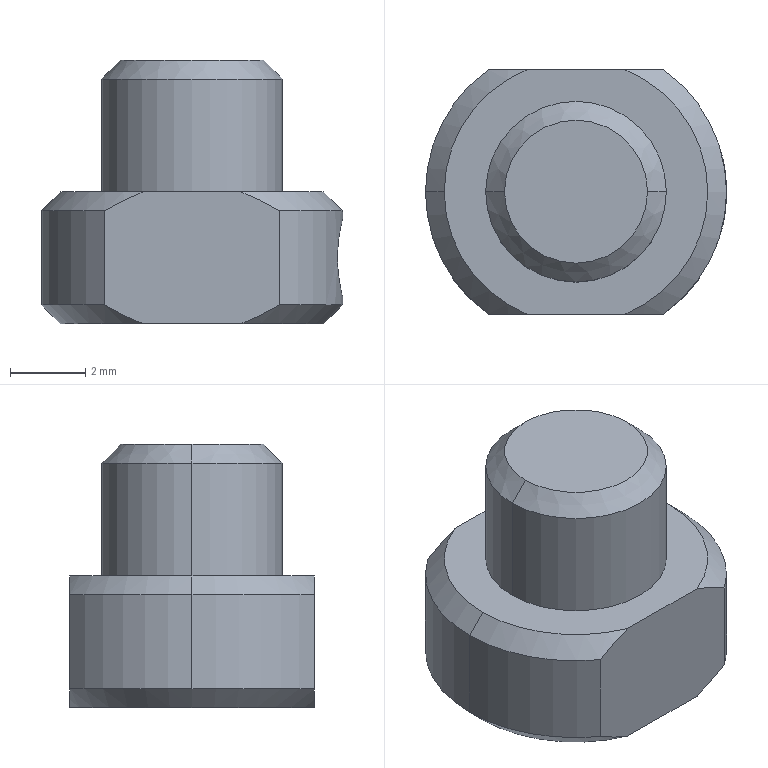Part | SolidWorks | features ICE 3, Chamfer 1, Extrusion 1, HoleWzd 1 | 1 solid | 23 faces | box 8 x 6.5 x 7 mm | volume 166.104 mm3 | cylinder 9 | cone 8 | plane 6 | commonest cylinder face diameters 8 x3 2.05 x2 3 x2 4.8 x2
STEP:
#1=CARTESIAN_POINT('',(1.9,0.,7.));
#2=VERTEX_POINT('',#1);
#3=CARTESIAN_POINT('',(-1.9,0.,7.));
#4=VERTEX_POINT('',#3);
#5=CARTESIAN_POINT('',(0.,0.,7.));
#6=DIRECTION('',(0.,0.,1.));
#7=DIRECTION('',(1.,0.,0.));
#8=AXIS2_PLACEMENT_3D('',#5,#6,#7);
#9=CIRCLE('',#8,1.9);
#10=EDGE_CURVE('',#2,#4,#9,.T.);
#11=ORIENTED_EDGE('',*,*,#10,.F.);
#12=CARTESIAN_POINT('',(2.4,0.,6.5));
#13=VERTEX_POINT('',#12);
#14=CARTESIAN_POINT('',(1.9,0.,7.));
#15=DIRECTION('',(0.7071,0.,-0.7071));
#16=VECTOR('',#15,1000.);
#17=LINE('',#14,#16);
#18=EDGE_CURVE('',#2,#13,#17,.T.);
#19=ORIENTED_EDGE('',*,*,#18,.T.);
#20=CARTESIAN_POINT('',(-2.4,0.,6.5));
#21=VERTEX_POINT('',#20);
#22=CARTESIAN_POINT('',(0.,0.,6.5));
#23=DIRECTION('',(0.,0.,-1.));
#24=DIRECTION('',(1.,0.,0.));
#25=AXIS2_PLACEMENT_3D('',#22,#23,#24);
#26=CIRCLE('',#25,2.4);
#27=EDGE_CURVE('',#21,#13,#26,.T.);
#28=ORIENTED_EDGE('',*,*,#27,.F.);
#29=CARTESIAN_POINT('',(-1.9,0.,7.));
#30=DIRECTION('',(-0.7071,0.,-0.7071));
#31=VECTOR('',#30,1000.);
#32=LINE('',#29,#31);
#33=EDGE_CURVE('',#4,#21,#32,.T.);
#34=ORIENTED_EDGE('',*,*,#33,.F.);
#35=EDGE_LOOP('',(#11,#19,#28,#34));
#36=FACE_OUTER_BOUND('',#35,.T.);
#37=CARTESIAN_POINT('',(0.,0.,7.));
#38=DIRECTION('',(0.,0.,-1.));
#39=DIRECTION('',(-1.,0.,0.));
#40=AXIS2_PLACEMENT_3D('',#37,#38,#39);
#41=CONICAL_SURFACE('',#40,1.9,0.7854);
#42=ADVANCED_FACE('',(#36),#41,.T.);
#43=CARTESIAN_POINT('',(1.5,0.,2.775));
#44=VERTEX_POINT('',#43);
#45=CARTESIAN_POINT('',(1.5,0.,0.725));
#46=VERTEX_POINT('',#45);
#47=CARTESIAN_POINT('',(1.5,0.,2.775));
#48=CARTESIAN_POINT('',(1.5,-0.1385,2.775));
#49=CARTESIAN_POINT('',(1.48,-0.2773,2.746));
#50=CARTESIAN_POINT('',(1.411,-0.5262,2.64));
#51=CARTESIAN_POINT('',(1.362,-0.6364,2.564));
#52=CARTESIAN_POINT('',(1.261,-0.8192,2.38));
#53=CARTESIAN_POINT('',(1.207,-0.8927,2.271));
#54=CARTESIAN_POINT('',(1.124,-0.9957,2.027));
#55=CARTESIAN_POINT('',(1.095,-1.025,1.889));
#56=CARTESIAN_POINT('',(1.095,-1.025,1.61));
#57=CARTESIAN_POINT('',(1.124,-0.9952,1.471));
#58=CARTESIAN_POINT('',(1.208,-0.8919,1.228));
#59=CARTESIAN_POINT('',(1.262,-0.8179,1.119));
#60=CARTESIAN_POINT('',(1.363,-0.6356,0.9355));
#61=CARTESIAN_POINT('',(1.411,-0.5254,0.8598));
#62=CARTESIAN_POINT('',(1.479,-0.2793,0.7548));
#63=CARTESIAN_POINT('',(1.5,-0.1404,0.725));
#64=CARTESIAN_POINT('',(1.5,0.,0.725));
#65=B_SPLINE_CURVE_WITH_KNOTS('',3,(#47,#48,#49,#50,#51,#52,#53,#54,#55,#56,#57,#58,#59,#60,#61,#62,#63,#64),.UNSPECIFIED.,.F.,.F.,(4,2,2,2,2,2,2,2,4),(0.003321,0.003736,0.00415,0.004565,0.004979,0.005394,0.005808,0.006223,0.006638),.UNSPECIFIED.);
#66=EDGE_CURVE('',#44,#46,#65,.T.);
#67=ORIENTED_EDGE('',*,*,#66,.F.);
#68=CARTESIAN_POINT('',(4.,0.,2.775));
#69=VERTEX_POINT('',#68);
#70=CARTESIAN_POINT('',(4.,0.,2.775));
#71=DIRECTION('',(1.,0.,0.));
#72=VECTOR('',#71,1000.);
#73=LINE('',#70,#72);
#74=EDGE_CURVE('',#44,#69,#73,.T.);
#75=ORIENTED_EDGE('',*,*,#74,.T.);
#76=CARTESIAN_POINT('',(4.,0.,0.725));
#77=VERTEX_POINT('',#76);
#78=CARTESIAN_POINT('',(4.,0.,0.725));
#79=CARTESIAN_POINT('',(4.,-0.1361,0.725));
#80=CARTESIAN_POINT('',(3.993,-0.2695,0.752));
#81=CARTESIAN_POINT('',(3.968,-0.5176,0.8551));
#82=CARTESIAN_POINT('',(3.951,-0.6309,0.9313));
#83=CARTESIAN_POINT('',(3.916,-0.8191,1.12));
#84=CARTESIAN_POINT('',(3.899,-0.8954,1.233));
#85=CARTESIAN_POINT('',(3.874,-0.9977,1.48));
#86=CARTESIAN_POINT('',(3.866,-1.025,1.615));
#87=CARTESIAN_POINT('',(3.866,-1.025,1.884));
#88=CARTESIAN_POINT('',(3.874,-0.9983,2.018));
#89=CARTESIAN_POINT('',(3.899,-0.895,2.267));
#90=CARTESIAN_POINT('',(3.916,-0.8196,2.38));
#91=CARTESIAN_POINT('',(3.951,-0.6297,2.57));
#92=CARTESIAN_POINT('',(3.968,-0.5167,2.645));
#93=CARTESIAN_POINT('',(3.993,-0.2692,2.748));
#94=CARTESIAN_POINT('',(4.,-0.1341,2.775));
#95=CARTESIAN_POINT('',(4.,0.,2.775));
#96=B_SPLINE_CURVE_WITH_KNOTS('',3,(#78,#79,#80,#81,#82,#83,#84,#85,#86,#87,#88,#89,#90,#91,#92,#93,#94,#95),.UNSPECIFIED.,.F.,.F.,(4,2,2,2,2,2,2,2,4),(0.,0.0004023,0.0008045,0.001207,0.001609,0.002011,0.002414,0.002816,0.003218),.UNSPECIFIED.);
#97=EDGE_CURVE('',#77,#69,#96,.T.);
#98=ORIENTED_EDGE('',*,*,#97,.F.);
#99=CARTESIAN_POINT('',(4.,0.,0.725));
#100=DIRECTION('',(1.,0.,0.));
#101=VECTOR('',#100,1000.);
#102=LINE('',#99,#101);
#103=EDGE_CURVE('',#46,#77,#102,.T.);
#104=ORIENTED_EDGE('',*,*,#103,.F.);
#105=EDGE_LOOP('',(#67,#75,#98,#104));
#106=FACE_OUTER_BOUND('',#105,.T.);
#107=CARTESIAN_POINT('',(4.,0.,1.75));
#108=DIRECTION('',(1.,0.,0.));
#109=DIRECTION('',(0.,0.,-1.));
#110=AXIS2_PLACEMENT_3D('',#107,#108,#109);
#111=CYLINDRICAL_SURFACE('',#110,1.025);
#112=ADVANCED_FACE('',(#106),#111,.F.);
#113=CARTESIAN_POINT('',(1.5,0.,6.));
#114=VERTEX_POINT('',#113);
#115=CARTESIAN_POINT('',(-1.5,0.,6.));
#116=VERTEX_POINT('',#115);
#117=CARTESIAN_POINT('',(0.,0.,6.));
#118=DIRECTION('',(0.,0.,-1.));
#119=DIRECTION('',(-1.,0.,0.));
#120=AXIS2_PLACEMENT_3D('',#117,#118,#119);
#121=CIRCLE('',#120,1.5);
#122=EDGE_CURVE('',#114,#116,#121,.T.);
#123=ORIENTED_EDGE('',*,*,#122,.F.);
#124=CARTESIAN_POINT('',(1.5,0.,6.));
#125=DIRECTION('',(0.,0.,-1.));
#126=VECTOR('',#125,1000.);
#127=LINE('',#124,#126);
#128=EDGE_CURVE('',#114,#44,#127,.T.);
#129=ORIENTED_EDGE('',*,*,#128,.T.);
#130=ORIENTED_EDGE('',*,*,#66,.T.);
#131=CARTESIAN_POINT('',(1.5,0.,0.));
#132=VERTEX_POINT('',#131);
#133=CARTESIAN_POINT('',(1.5,0.,6.));
#134=DIRECTION('',(0.,0.,-1.));
#135=VECTOR('',#134,1000.);
#136=LINE('',#133,#135);
#137=EDGE_CURVE('',#46,#132,#136,.T.);
#138=ORIENTED_EDGE('',*,*,#137,.T.);
#139=CARTESIAN_POINT('',(-1.5,0.,0.));
#140=VERTEX_POINT('',#139);
#141=CARTESIAN_POINT('',(0.,0.,0.));
#142=DIRECTION('',(0.,0.,-1.));
#143=DIRECTION('',(-1.,0.,0.));
#144=AXIS2_PLACEMENT_3D('',#141,#142,#143);
#145=CIRCLE('',#144,1.5);
#146=EDGE_CURVE('',#132,#140,#145,.T.);
#147=ORIENTED_EDGE('',*,*,#146,.T.);
#148=CARTESIAN_POINT('',(-1.5,0.,6.));
#149=DIRECTION('',(0.,0.,-1.));
#150=VECTOR('',#149,1000.);
#151=LINE('',#148,#150);
#152=EDGE_CURVE('',#116,#140,#151,.T.);
#153=ORIENTED_EDGE('',*,*,#152,.F.);
#154=EDGE_LOOP('',(#123,#129,#130,#138,#147,#153));
#155=FACE_OUTER_BOUND('',#154,.T.);
#156=CARTESIAN_POINT('',(0.,0.,6.));
#157=DIRECTION('',(0.,0.,-1.));
#158=DIRECTION('',(-1.,0.,0.));
#159=AXIS2_PLACEMENT_3D('',#156,#157,#158);
#160=CYLINDRICAL_SURFACE('',#159,1.5);
#161=ADVANCED_FACE('',(#155),#160,.F.);
#162=ORIENTED_EDGE('',*,*,#27,.T.);
#163=CARTESIAN_POINT('',(2.4,0.,3.5));
#164=VERTEX_POINT('',#163);
#165=CARTESIAN_POINT('',(2.4,0.,7.));
#166=DIRECTION('',(0.,0.,-1.));
#167=VECTOR('',#166,1000.);
#168=LINE('',#165,#167);
#169=EDGE_CURVE('',#13,#164,#168,.T.);
#170=ORIENTED_EDGE('',*,*,#169,.T.);
#171=CARTESIAN_POINT('',(-2.4,0.,3.5));
#172=VERTEX_POINT('',#171);
#173=CARTESIAN_POINT('',(0.,0.,3.5));
#174=DIRECTION('',(0.,0.,1.));
#175=DIRECTION('',(1.,0.,0.));
#176=AXIS2_PLACEMENT_3D('',#173,#174,#175);
#177=CIRCLE('',#176,2.4);
#178=EDGE_CURVE('',#164,#172,#177,.T.);
#179=ORIENTED_EDGE('',*,*,#178,.T.);
#180=CARTESIAN_POINT('',(-2.4,0.,7.));
#181=DIRECTION('',(0.,0.,-1.));
#182=VECTOR('',#181,1000.);
#183=LINE('',#180,#182);
#184=EDGE_CURVE('',#21,#172,#183,.T.);
#185=ORIENTED_EDGE('',*,*,#184,.F.);
#186=EDGE_LOOP('',(#162,#170,#179,#185));
#187=FACE_OUTER_BOUND('',#186,.T.);
#188=CARTESIAN_POINT('',(0.,0.,7.));
#189=DIRECTION('',(0.,0.,-1.));
#190=DIRECTION('',(-1.,0.,0.));
#191=AXIS2_PLACEMENT_3D('',#188,#189,#190);
#192=CYLINDRICAL_SURFACE('',#191,2.4);
#193=ADVANCED_FACE('',(#187),#192,.T.);
#194=CARTESIAN_POINT('',(3.5,0.,0.));
#195=VERTEX_POINT('',#194);
#196=CARTESIAN_POINT('',(1.299,-3.25,0.));
#197=VERTEX_POINT('',#196);
#198=CARTESIAN_POINT('',(0.,0.,0.));
#199=DIRECTION('',(0.,0.,-1.));
#200=DIRECTION('',(1.,0.,0.));
#201=AXIS2_PLACEMENT_3D('',#198,#199,#200);
#202=CIRCLE('',#201,3.5);
#203=EDGE_CURVE('',#195,#197,#202,.T.);
#204=ORIENTED_EDGE('',*,*,#203,.F.);
#205=CARTESIAN_POINT('',(4.,0.,0.5));
#206=VERTEX_POINT('',#205);
#207=CARTESIAN_POINT('',(4.,0.,0.5));
#208=DIRECTION('',(0.7071,0.,0.7071));
#209=VECTOR('',#208,1000.);
#210=LINE('',#207,#209);
#211=EDGE_CURVE('',#195,#206,#210,.T.);
#212=ORIENTED_EDGE('',*,*,#211,.T.);
#213=CARTESIAN_POINT('',(2.332,-3.25,0.5));
#214=VERTEX_POINT('',#213);
#215=CARTESIAN_POINT('',(0.,0.,0.5));
#216=DIRECTION('',(0.,0.,1.));
#217=DIRECTION('',(1.,0.,0.));
#218=AXIS2_PLACEMENT_3D('',#215,#216,#217);
#219=CIRCLE('',#218,4.);
#220=EDGE_CURVE('',#214,#206,#219,.T.);
#221=ORIENTED_EDGE('',*,*,#220,.F.);
#222=CARTESIAN_POINT('',(2.332,-3.25,0.5));
#223=CARTESIAN_POINT('',(2.001,-3.25,0.3069));
#224=CARTESIAN_POINT('',(1.659,-3.25,0.1338));
#225=CARTESIAN_POINT('',(1.299,-3.25,0.));
#226=B_SPLINE_CURVE_WITH_KNOTS('',3,(#222,#223,#224,#225),.UNSPECIFIED.,.F.,.F.,(4,4),(0.007591,0.00874),.UNSPECIFIED.);
#227=EDGE_CURVE('',#214,#197,#226,.T.);
#228=ORIENTED_EDGE('',*,*,#227,.T.);
#229=EDGE_LOOP('',(#204,#212,#221,#228));
#230=FACE_OUTER_BOUND('',#229,.T.);
#231=CARTESIAN_POINT('',(0.,0.,0.5));
#232=DIRECTION('',(0.,0.,1.));
#233=DIRECTION('',(1.,0.,0.));
#234=AXIS2_PLACEMENT_3D('',#231,#232,#233);
#235=CONICAL_SURFACE('',#234,4.,0.7854);
#236=ADVANCED_FACE('',(#230),#235,.T.);
#237=CARTESIAN_POINT('',(-3.5,0.,3.5));
#238=VERTEX_POINT('',#237);
#239=CARTESIAN_POINT('',(-1.299,-3.25,3.5));
#240=VERTEX_POINT('',#239);
#241=CARTESIAN_POINT('',(0.,0.,3.5));
#242=DIRECTION('',(0.,0.,1.));
#243=DIRECTION('',(1.,0.,0.));
#244=AXIS2_PLACEMENT_3D('',#241,#242,#243);
#245=CIRCLE('',#244,3.5);
#246=EDGE_CURVE('',#238,#240,#245,.T.);
#247=ORIENTED_EDGE('',*,*,#246,.F.);
#248=CARTESIAN_POINT('',(-4.,0.,3.));
#249=VERTEX_POINT('',#248);
#250=CARTESIAN_POINT('',(-3.5,0.,3.5));
#251=DIRECTION('',(-0.7071,0.,-0.7071));
#252=VECTOR('',#251,1000.);
#253=LINE('',#250,#252);
#254=EDGE_CURVE('',#238,#249,#253,.T.);
#255=ORIENTED_EDGE('',*,*,#254,.T.);
#256=CARTESIAN_POINT('',(-2.332,-3.25,3.));
#257=VERTEX_POINT('',#256);
#258=CARTESIAN_POINT('',(0.,0.,3.));
#259=DIRECTION('',(0.,0.,-1.));
#260=DIRECTION('',(1.,0.,0.));
#261=AXIS2_PLACEMENT_3D('',#258,#259,#260);
#262=CIRCLE('',#261,4.);
#263=EDGE_CURVE('',#257,#249,#262,.T.);
#264=ORIENTED_EDGE('',*,*,#263,.F.);
#265=CARTESIAN_POINT('',(-2.332,-3.25,3.));
#266=CARTESIAN_POINT('',(-2.001,-3.25,3.193));
#267=CARTESIAN_POINT('',(-1.659,-3.25,3.366));
#268=CARTESIAN_POINT('',(-1.299,-3.25,3.5));
#269=B_SPLINE_CURVE_WITH_KNOTS('',3,(#265,#266,#267,#268),.UNSPECIFIED.,.F.,.F.,(4,4),(0.007591,0.00874),.UNSPECIFIED.);
#270=EDGE_CURVE('',#257,#240,#269,.T.);
#271=ORIENTED_EDGE('',*,*,#270,.T.);
#272=EDGE_LOOP('',(#247,#255,#264,#271));
#273=FACE_OUTER_BOUND('',#272,.T.);
#274=CARTESIAN_POINT('',(0.,0.,3.5));
#275=DIRECTION('',(0.,0.,-1.));
#276=DIRECTION('',(-1.,0.,0.));
#277=AXIS2_PLACEMENT_3D('',#274,#275,#276);
#278=CONICAL_SURFACE('',#277,3.5,0.7854);
#279=ADVANCED_FACE('',(#273),#278,.T.);
#280=ORIENTED_EDGE('',*,*,#263,.T.);
#281=CARTESIAN_POINT('',(-4.,0.,0.5));
#282=VERTEX_POINT('',#281);
#283=CARTESIAN_POINT('',(-4.,0.,3.5));
#284=DIRECTION('',(0.,0.,-1.));
#285=VECTOR('',#284,1000.);
#286=LINE('',#283,#285);
#287=EDGE_CURVE('',#249,#282,#286,.T.);
#288=ORIENTED_EDGE('',*,*,#287,.T.);
#289=CARTESIAN_POINT('',(-2.332,-3.25,0.5));
#290=VERTEX_POINT('',#289);
#291=CARTESIAN_POINT('',(0.,0.,0.5));
#292=DIRECTION('',(0.,0.,1.));
#293=DIRECTION('',(1.,0.,0.));
#294=AXIS2_PLACEMENT_3D('',#291,#292,#293);
#295=CIRCLE('',#294,4.);
#296=EDGE_CURVE('',#282,#290,#295,.T.);
#297=ORIENTED_EDGE('',*,*,#296,.T.);
#298=CARTESIAN_POINT('',(-2.332,-3.25,3.5));
#299=DIRECTION('',(0.,0.,-1.));
#300=VECTOR('',#299,1000.);
#301=LINE('',#298,#300);
#302=EDGE_CURVE('',#257,#290,#301,.T.);
#303=ORIENTED_EDGE('',*,*,#302,.F.);
#304=EDGE_LOOP('',(#280,#288,#297,#303));
#305=FACE_OUTER_BOUND('',#304,.T.);
#306=CARTESIAN_POINT('',(0.,0.,3.5));
#307=DIRECTION('',(0.,0.,-1.));
#308=DIRECTION('',(-1.,0.,0.));
#309=AXIS2_PLACEMENT_3D('',#306,#307,#308);
#310=CYLINDRICAL_SURFACE('',#309,4.);
#311=ADVANCED_FACE('',(#305),#310,.T.);
#312=CARTESIAN_POINT('',(0.,0.,3.5));
#313=DIRECTION('',(0.,0.,1.));
#314=DIRECTION('',(1.,0.,0.));
#315=AXIS2_PLACEMENT_3D('',#312,#313,#314);
#316=CIRCLE('',#315,2.4);
#317=EDGE_CURVE('',#172,#164,#316,.T.);
#318=ORIENTED_EDGE('',*,*,#317,.F.);
#319=ORIENTED_EDGE('',*,*,#178,.F.);
#320=EDGE_LOOP('',(#318,#319));
#321=FACE_BOUND('',#320,.T.);
#322=CARTESIAN_POINT('',(-1.299,3.25,3.5));
#323=VERTEX_POINT('',#322);
#324=CARTESIAN_POINT('',(0.,0.,3.5));
#325=DIRECTION('',(0.,0.,1.));
#326=DIRECTION('',(1.,0.,0.));
#327=AXIS2_PLACEMENT_3D('',#324,#325,#326);
#328=CIRCLE('',#327,3.5);
#329=EDGE_CURVE('',#323,#238,#328,.T.);
#330=ORIENTED_EDGE('',*,*,#329,.T.);
#331=ORIENTED_EDGE('',*,*,#246,.T.);
#332=CARTESIAN_POINT('',(1.299,-3.25,3.5));
#333=VERTEX_POINT('',#332);
#334=CARTESIAN_POINT('',(-5.597,-3.25,3.5));
#335=DIRECTION('',(1.,0.,0.));
#336=VECTOR('',#335,1000.);
#337=LINE('',#334,#336);
#338=EDGE_CURVE('',#240,#333,#337,.T.);
#339=ORIENTED_EDGE('',*,*,#338,.T.);
#340=CARTESIAN_POINT('',(1.299,3.25,3.5));
#341=VERTEX_POINT('',#340);
#342=CARTESIAN_POINT('',(0.,0.,3.5));
#343=DIRECTION('',(0.,0.,1.));
#344=DIRECTION('',(1.,0.,0.));
#345=AXIS2_PLACEMENT_3D('',#342,#343,#344);
#346=CIRCLE('',#345,3.5);
#347=EDGE_CURVE('',#333,#341,#346,.T.);
#348=ORIENTED_EDGE('',*,*,#347,.T.);
#349=CARTESIAN_POINT('',(-5.597,3.25,3.5));
#350=DIRECTION('',(-1.,0.,0.));
#351=VECTOR('',#350,1000.);
#352=LINE('',#349,#351);
#353=EDGE_CURVE('',#341,#323,#352,.T.);
#354=ORIENTED_EDGE('',*,*,#353,.T.);
#355=EDGE_LOOP('',(#330,#331,#339,#348,#354));
#356=FACE_OUTER_BOUND('',#355,.T.);
#357=CARTESIAN_POINT('',(0.,0.,3.5));
#358=DIRECTION('',(0.,0.,1.));
#359=DIRECTION('',(1.,0.,0.));
#360=AXIS2_PLACEMENT_3D('',#357,#358,#359);
#361=PLANE('',#360);
#362=ADVANCED_FACE('',(#321,#356),#361,.T.);
#363=ORIENTED_EDGE('',*,*,#287,.F.);
#364=CARTESIAN_POINT('',(-2.332,3.25,3.));
#365=VERTEX_POINT('',#364);
#366=CARTESIAN_POINT('',(0.,0.,3.));
#367=DIRECTION('',(0.,0.,-1.));
#368=DIRECTION('',(1.,0.,0.));
#369=AXIS2_PLACEMENT_3D('',#366,#367,#368);
#370=CIRCLE('',#369,4.);
#371=EDGE_CURVE('',#249,#365,#370,.T.);
#372=ORIENTED_EDGE('',*,*,#371,.T.);
#373=CARTESIAN_POINT('',(-2.332,3.25,0.5));
#374=VERTEX_POINT('',#373);
#375=CARTESIAN_POINT('',(-2.332,3.25,3.5));
#376=DIRECTION('',(0.,0.,1.));
#377=VECTOR('',#376,1000.);
#378=LINE('',#375,#377);
#379=EDGE_CURVE('',#374,#365,#378,.T.);
#380=ORIENTED_EDGE('',*,*,#379,.F.);
#381=CARTESIAN_POINT('',(0.,0.,0.5));
#382=DIRECTION('',(0.,0.,1.));
#383=DIRECTION('',(1.,0.,0.));
#384=AXIS2_PLACEMENT_3D('',#381,#382,#383);
#385=CIRCLE('',#384,4.);
#386=EDGE_CURVE('',#374,#282,#385,.T.);
#387=ORIENTED_EDGE('',*,*,#386,.T.);
#388=EDGE_LOOP('',(#363,#372,#380,#387));
#389=FACE_OUTER_BOUND('',#388,.T.);
#390=CARTESIAN_POINT('',(0.,0.,3.5));
#391=DIRECTION('',(0.,0.,-1.));
#392=DIRECTION('',(-1.,0.,0.));
#393=AXIS2_PLACEMENT_3D('',#390,#391,#392);
#394=CYLINDRICAL_SURFACE('',#393,4.);
#395=ADVANCED_FACE('',(#389),#394,.T.);
#396=ORIENTED_EDGE('',*,*,#97,.T.);
#397=CARTESIAN_POINT('',(4.,0.,2.775));
#398=CARTESIAN_POINT('',(4.,0.1341,2.775));
#399=CARTESIAN_POINT('',(3.993,0.2695,2.748));
#400=CARTESIAN_POINT('',(3.968,0.5164,2.645));
#401=CARTESIAN_POINT('',(3.951,0.63,2.57));
#402=CARTESIAN_POINT('',(3.916,0.8191,2.381));
#403=CARTESIAN_POINT('',(3.899,0.8945,2.268));
#404=CARTESIAN_POINT('',(3.874,0.9983,2.019));
#405=CARTESIAN_POINT('',(3.866,1.025,1.885));
#406=CARTESIAN_POINT('',(3.866,1.025,1.615));
#407=CARTESIAN_POINT('',(3.874,0.998,1.481));
#408=CARTESIAN_POINT('',(3.899,0.8954,1.233));
#409=CARTESIAN_POINT('',(3.916,0.8192,1.12));
#410=CARTESIAN_POINT('',(3.951,0.6312,0.9315));
#411=CARTESIAN_POINT('',(3.968,0.5175,0.8552));
#412=CARTESIAN_POINT('',(3.993,0.2707,0.7524));
#413=CARTESIAN_POINT('',(4.,0.136,0.725));
#414=CARTESIAN_POINT('',(4.,0.,0.725));
#415=B_SPLINE_CURVE_WITH_KNOTS('',3,(#397,#398,#399,#400,#401,#402,#403,#404,#405,#406,#407,#408,#409,#410,#411,#412,#413,#414),.UNSPECIFIED.,.F.,.F.,(4,2,2,2,2,2,2,2,4),(0.003218,0.00362,0.004022,0.004425,0.004827,0.005229,0.005631,0.006033,0.006435),.UNSPECIFIED.);
#416=EDGE_CURVE('',#69,#77,#415,.T.);
#417=ORIENTED_EDGE('',*,*,#416,.T.);
#418=EDGE_LOOP('',(#396,#417));
#419=FACE_BOUND('',#418,.T.);
#420=CARTESIAN_POINT('',(2.332,-3.25,3.));
#421=VERTEX_POINT('',#420);
#422=CARTESIAN_POINT('',(2.332,-3.25,3.5));
#423=DIRECTION('',(0.,0.,1.));
#424=VECTOR('',#423,1000.);
#425=LINE('',#422,#424);
#426=EDGE_CURVE('',#214,#421,#425,.T.);
#427=ORIENTED_EDGE('',*,*,#426,.F.);
#428=ORIENTED_EDGE('',*,*,#220,.T.);
#429=CARTESIAN_POINT('',(2.332,3.25,0.5));
#430=VERTEX_POINT('',#429);
#431=CARTESIAN_POINT('',(0.,0.,0.5));
#432=DIRECTION('',(0.,0.,1.));
#433=DIRECTION('',(1.,0.,0.));
#434=AXIS2_PLACEMENT_3D('',#431,#432,#433);
#435=CIRCLE('',#434,4.);
#436=EDGE_CURVE('',#206,#430,#435,.T.);
#437=ORIENTED_EDGE('',*,*,#436,.T.);
#438=CARTESIAN_POINT('',(2.332,3.25,3.));
#439=VERTEX_POINT('',#438);
#440=CARTESIAN_POINT('',(2.332,3.25,3.5));
#441=DIRECTION('',(0.,0.,-1.));
#442=VECTOR('',#441,1000.);
#443=LINE('',#440,#442);
#444=EDGE_CURVE('',#439,#430,#443,.T.);
#445=ORIENTED_EDGE('',*,*,#444,.F.);
#446=CARTESIAN_POINT('',(0.,0.,3.));
#447=DIRECTION('',(0.,0.,-1.));
#448=DIRECTION('',(1.,0.,0.));
#449=AXIS2_PLACEMENT_3D('',#446,#447,#448);
#450=CIRCLE('',#449,4.);
#451=EDGE_CURVE('',#439,#421,#450,.T.);
#452=ORIENTED_EDGE('',*,*,#451,.T.);
#453=EDGE_LOOP('',(#427,#428,#437,#445,#452));
#454=FACE_OUTER_BOUND('',#453,.T.);
#455=CARTESIAN_POINT('',(0.,0.,3.5));
#456=DIRECTION('',(0.,0.,-1.));
#457=DIRECTION('',(-1.,0.,0.));
#458=AXIS2_PLACEMENT_3D('',#455,#456,#457);
#459=CYLINDRICAL_SURFACE('',#458,4.);
#460=ADVANCED_FACE('',(#419,#454),#459,.T.);
#461=CARTESIAN_POINT('',(0.,0.,0.));
#462=DIRECTION('',(0.,0.,-1.));
#463=DIRECTION('',(-1.,0.,0.));
#464=AXIS2_PLACEMENT_3D('',#461,#462,#463);
#465=CIRCLE('',#464,1.5);
#466=EDGE_CURVE('',#140,#132,#465,.T.);
#467=ORIENTED_EDGE('',*,*,#466,.F.);
#468=ORIENTED_EDGE('',*,*,#146,.F.);
#469=EDGE_LOOP('',(#467,#468));
#470=FACE_BOUND('',#469,.T.);
#471=CARTESIAN_POINT('',(-1.299,-3.25,0.));
#472=VERTEX_POINT('',#471);
#473=CARTESIAN_POINT('',(0.,-3.25,0.));
#474=DIRECTION('',(1.,0.,0.));
#475=VECTOR('',#474,1000.);
#476=LINE('',#473,#475);
#477=EDGE_CURVE('',#472,#197,#476,.T.);
#478=ORIENTED_EDGE('',*,*,#477,.F.);
#479=CARTESIAN_POINT('',(-1.299,3.25,0.));
#480=VERTEX_POINT('',#479);
#481=CARTESIAN_POINT('',(0.,0.,0.));
#482=DIRECTION('',(0.,0.,-1.));
#483=DIRECTION('',(1.,0.,0.));
#484=AXIS2_PLACEMENT_3D('',#481,#482,#483);
#485=CIRCLE('',#484,3.5);
#486=EDGE_CURVE('',#472,#480,#485,.T.);
#487=ORIENTED_EDGE('',*,*,#486,.T.);
#488=CARTESIAN_POINT('',(1.299,3.25,0.));
#489=VERTEX_POINT('',#488);
#490=CARTESIAN_POINT('',(0.,3.25,0.));
#491=DIRECTION('',(-1.,0.,0.));
#492=VECTOR('',#491,1000.);
#493=LINE('',#490,#492);
#494=EDGE_CURVE('',#489,#480,#493,.T.);
#495=ORIENTED_EDGE('',*,*,#494,.F.);
#496=CARTESIAN_POINT('',(0.,0.,0.));
#497=DIRECTION('',(0.,0.,-1.));
#498=DIRECTION('',(1.,0.,0.));
#499=AXIS2_PLACEMENT_3D('',#496,#497,#498);
#500=CIRCLE('',#499,3.5);
#501=EDGE_CURVE('',#489,#195,#500,.T.);
#502=ORIENTED_EDGE('',*,*,#501,.T.);
#503=ORIENTED_EDGE('',*,*,#203,.T.);
#504=EDGE_LOOP('',(#478,#487,#495,#502,#503));
#505=FACE_OUTER_BOUND('',#504,.T.);
#506=CARTESIAN_POINT('',(0.,0.,0.));
#507=DIRECTION('',(0.,0.,1.));
#508=DIRECTION('',(1.,0.,0.));
#509=AXIS2_PLACEMENT_3D('',#506,#507,#508);
#510=PLANE('',#509);
#511=ADVANCED_FACE('',(#470,#505),#510,.F.);
#512=ORIENTED_EDGE('',*,*,#254,.F.);
#513=ORIENTED_EDGE('',*,*,#329,.F.);
#514=CARTESIAN_POINT('',(-1.299,3.25,3.5));
#515=CARTESIAN_POINT('',(-1.662,3.25,3.365));
#516=CARTESIAN_POINT('',(-2.002,3.25,3.192));
#517=CARTESIAN_POINT('',(-2.332,3.25,3.));
#518=B_SPLINE_CURVE_WITH_KNOTS('',3,(#514,#515,#516,#517),.UNSPECIFIED.,.F.,.F.,(4,4),(0.0114,0.01256),.UNSPECIFIED.);
#519=EDGE_CURVE('',#323,#365,#518,.T.);
#520=ORIENTED_EDGE('',*,*,#519,.T.);
#521=ORIENTED_EDGE('',*,*,#371,.F.);
#522=EDGE_LOOP('',(#512,#513,#520,#521));
#523=FACE_OUTER_BOUND('',#522,.T.);
#524=CARTESIAN_POINT('',(0.,0.,3.5));
#525=DIRECTION('',(0.,0.,-1.));
#526=DIRECTION('',(-1.,0.,0.));
#527=AXIS2_PLACEMENT_3D('',#524,#525,#526);
#528=CONICAL_SURFACE('',#527,3.5,0.7854);
#529=ADVANCED_FACE('',(#523),#528,.T.);
#530=ORIENTED_EDGE('',*,*,#347,.F.);
#531=CARTESIAN_POINT('',(1.299,-3.25,3.5));
#532=CARTESIAN_POINT('',(1.662,-3.25,3.365));
#533=CARTESIAN_POINT('',(2.002,-3.25,3.192));
#534=CARTESIAN_POINT('',(2.332,-3.25,3.));
#535=B_SPLINE_CURVE_WITH_KNOTS('',3,(#531,#532,#533,#534),.UNSPECIFIED.,.F.,.F.,(4,4),(0.0114,0.01256),.UNSPECIFIED.);
#536=EDGE_CURVE('',#333,#421,#535,.T.);
#537=ORIENTED_EDGE('',*,*,#536,.T.);
#538=ORIENTED_EDGE('',*,*,#451,.F.);
#539=CARTESIAN_POINT('',(2.332,3.25,3.));
#540=CARTESIAN_POINT('',(2.001,3.25,3.193));
#541=CARTESIAN_POINT('',(1.659,3.25,3.366));
#542=CARTESIAN_POINT('',(1.299,3.25,3.5));
#543=B_SPLINE_CURVE_WITH_KNOTS('',3,(#539,#540,#541,#542),.UNSPECIFIED.,.F.,.F.,(4,4),(0.007591,0.00874),.UNSPECIFIED.);
#544=EDGE_CURVE('',#439,#341,#543,.T.);
#545=ORIENTED_EDGE('',*,*,#544,.T.);
#546=EDGE_LOOP('',(#530,#537,#538,#545));
#547=FACE_OUTER_BOUND('',#546,.T.);
#548=CARTESIAN_POINT('',(0.,0.,3.5));
#549=DIRECTION('',(0.,0.,-1.));
#550=DIRECTION('',(-1.,0.,0.));
#551=AXIS2_PLACEMENT_3D('',#548,#549,#550);
#552=CONICAL_SURFACE('',#551,3.5,0.7854);
#553=ADVANCED_FACE('',(#547),#552,.T.);
#554=ORIENTED_EDGE('',*,*,#211,.F.);
#555=ORIENTED_EDGE('',*,*,#501,.F.);
#556=CARTESIAN_POINT('',(1.299,3.25,0.));
#557=CARTESIAN_POINT('',(1.662,3.25,0.1346));
#558=CARTESIAN_POINT('',(2.002,3.25,0.3078));
#559=CARTESIAN_POINT('',(2.332,3.25,0.5));
#560=B_SPLINE_CURVE_WITH_KNOTS('',3,(#556,#557,#558,#559),.UNSPECIFIED.,.F.,.F.,(4,4),(0.0114,0.01256),.UNSPECIFIED.);
#561=EDGE_CURVE('',#489,#430,#560,.T.);
#562=ORIENTED_EDGE('',*,*,#561,.T.);
#563=ORIENTED_EDGE('',*,*,#436,.F.);
#564=EDGE_LOOP('',(#554,#555,#562,#563));
#565=FACE_OUTER_BOUND('',#564,.T.);
#566=CARTESIAN_POINT('',(0.,0.,0.5));
#567=DIRECTION('',(0.,0.,1.));
#568=DIRECTION('',(1.,0.,0.));
#569=AXIS2_PLACEMENT_3D('',#566,#567,#568);
#570=CONICAL_SURFACE('',#569,4.,0.7854);
#571=ADVANCED_FACE('',(#565),#570,.T.);
#572=ORIENTED_EDGE('',*,*,#486,.F.);
#573=CARTESIAN_POINT('',(-1.299,-3.25,0.));
#574=CARTESIAN_POINT('',(-1.662,-3.25,0.1346));
#575=CARTESIAN_POINT('',(-2.002,-3.25,0.3078));
#576=CARTESIAN_POINT('',(-2.332,-3.25,0.5));
#577=B_SPLINE_CURVE_WITH_KNOTS('',3,(#573,#574,#575,#576),.UNSPECIFIED.,.F.,.F.,(4,4),(0.0114,0.01256),.UNSPECIFIED.);
#578=EDGE_CURVE('',#472,#290,#577,.T.);
#579=ORIENTED_EDGE('',*,*,#578,.T.);
#580=ORIENTED_EDGE('',*,*,#296,.F.);
#581=ORIENTED_EDGE('',*,*,#386,.F.);
#582=CARTESIAN_POINT('',(-2.332,3.25,0.5));
#583=CARTESIAN_POINT('',(-2.001,3.25,0.3069));
#584=CARTESIAN_POINT('',(-1.659,3.25,0.1338));
#585=CARTESIAN_POINT('',(-1.299,3.25,0.));
#586=B_SPLINE_CURVE_WITH_KNOTS('',3,(#582,#583,#584,#585),.UNSPECIFIED.,.F.,.F.,(4,4),(0.007591,0.00874),.UNSPECIFIED.);
#587=EDGE_CURVE('',#374,#480,#586,.T.);
#588=ORIENTED_EDGE('',*,*,#587,.T.);
#589=EDGE_LOOP('',(#572,#579,#580,#581,#588));
#590=FACE_OUTER_BOUND('',#589,.T.);
#591=CARTESIAN_POINT('',(0.,0.,0.5));
#592=DIRECTION('',(0.,0.,1.));
#593=DIRECTION('',(1.,0.,0.));
#594=AXIS2_PLACEMENT_3D('',#591,#592,#593);
#595=CONICAL_SURFACE('',#594,4.,0.7854);
#596=ADVANCED_FACE('',(#590),#595,.T.);
#597=ORIENTED_EDGE('',*,*,#169,.F.);
#598=CARTESIAN_POINT('',(0.,0.,6.5));
#599=DIRECTION('',(0.,0.,-1.));
#600=DIRECTION('',(1.,0.,0.));
#601=AXIS2_PLACEMENT_3D('',#598,#599,#600);
#602=CIRCLE('',#601,2.4);
#603=EDGE_CURVE('',#13,#21,#602,.T.);
#604=ORIENTED_EDGE('',*,*,#603,.T.);
#605=ORIENTED_EDGE('',*,*,#184,.T.);
#606=ORIENTED_EDGE('',*,*,#317,.T.);
#607=EDGE_LOOP('',(#597,#604,#605,#606));
#608=FACE_OUTER_BOUND('',#607,.T.);
#609=CARTESIAN_POINT('',(0.,0.,7.));
#610=DIRECTION('',(0.,0.,-1.));
#611=DIRECTION('',(-1.,0.,0.));
#612=AXIS2_PLACEMENT_3D('',#609,#610,#611);
#613=CYLINDRICAL_SURFACE('',#612,2.4);
#614=ADVANCED_FACE('',(#608),#613,.T.);
#615=CARTESIAN_POINT('',(0.,0.,7.));
#616=DIRECTION('',(0.,0.,1.));
#617=DIRECTION('',(1.,0.,0.));
#618=AXIS2_PLACEMENT_3D('',#615,#616,#617);
#619=CIRCLE('',#618,1.9);
#620=EDGE_CURVE('',#4,#2,#619,.T.);
#621=ORIENTED_EDGE('',*,*,#620,.T.);
#622=ORIENTED_EDGE('',*,*,#10,.T.);
#623=EDGE_LOOP('',(#621,#622));
#624=FACE_OUTER_BOUND('',#623,.T.);
#625=CARTESIAN_POINT('',(0.,0.,7.));
#626=DIRECTION('',(0.,0.,1.));
#627=DIRECTION('',(1.,0.,0.));
#628=AXIS2_PLACEMENT_3D('',#625,#626,#627);
#629=PLANE('',#628);
#630=ADVANCED_FACE('',(#624),#629,.T.);
#631=ORIENTED_EDGE('',*,*,#128,.F.);
#632=CARTESIAN_POINT('',(0.,0.,6.));
#633=DIRECTION('',(0.,0.,-1.));
#634=DIRECTION('',(-1.,0.,0.));
#635=AXIS2_PLACEMENT_3D('',#632,#633,#634);
#636=CIRCLE('',#635,1.5);
#637=EDGE_CURVE('',#116,#114,#636,.T.);
#638=ORIENTED_EDGE('',*,*,#637,.F.);
#639=ORIENTED_EDGE('',*,*,#152,.T.);
#640=ORIENTED_EDGE('',*,*,#466,.T.);
#641=ORIENTED_EDGE('',*,*,#137,.F.);
#642=CARTESIAN_POINT('',(1.5,0.,0.725));
#643=CARTESIAN_POINT('',(1.5,0.1406,0.725));
#644=CARTESIAN_POINT('',(1.48,0.2781,0.7543));
#645=CARTESIAN_POINT('',(1.411,0.5256,0.8598));
#646=CARTESIAN_POINT('',(1.363,0.6359,0.9358));
#647=CARTESIAN_POINT('',(1.261,0.8184,1.119));
#648=CARTESIAN_POINT('',(1.208,0.8918,1.228));
#649=CARTESIAN_POINT('',(1.124,0.9953,1.472));
#650=CARTESIAN_POINT('',(1.095,1.025,1.61));
#651=CARTESIAN_POINT('',(1.095,1.025,1.889));
#652=CARTESIAN_POINT('',(1.124,0.996,2.027));
#653=CARTESIAN_POINT('',(1.208,0.8921,2.272));
#654=CARTESIAN_POINT('',(1.261,0.8193,2.38));
#655=CARTESIAN_POINT('',(1.363,0.6355,2.565));
#656=CARTESIAN_POINT('',(1.41,0.5275,2.639));
#657=CARTESIAN_POINT('',(1.462,0.3399,2.719));
#658=CARTESIAN_POINT('',(1.476,0.2749,2.74));
#659=CARTESIAN_POINT('',(1.495,0.1398,2.768));
#660=CARTESIAN_POINT('',(1.5,0.06933,2.775));
#661=CARTESIAN_POINT('',(1.5,0.,2.775));
#662=B_SPLINE_CURVE_WITH_KNOTS('',3,(#642,#643,#644,#645,#646,#647,#648,#649,#650,#651,#652,#653,#654,#655,#656,#657,#658,#659,#660,#661),.UNSPECIFIED.,.F.,.F.,(4,2,2,2,2,2,2,2,2,4),(0.,0.0004152,0.0008303,0.001245,0.001661,0.002076,0.002491,0.002906,0.003114,0.003321),.UNSPECIFIED.);
#663=EDGE_CURVE('',#46,#44,#662,.T.);
#664=ORIENTED_EDGE('',*,*,#663,.T.);
#665=EDGE_LOOP('',(#631,#638,#639,#640,#641,#664));
#666=FACE_OUTER_BOUND('',#665,.T.);
#667=CARTESIAN_POINT('',(0.,0.,6.));
#668=DIRECTION('',(0.,0.,-1.));
#669=DIRECTION('',(-1.,0.,0.));
#670=AXIS2_PLACEMENT_3D('',#667,#668,#669);
#671=CYLINDRICAL_SURFACE('',#670,1.5);
#672=ADVANCED_FACE('',(#666),#671,.F.);
#673=ORIENTED_EDGE('',*,*,#637,.T.);
#674=ORIENTED_EDGE('',*,*,#122,.T.);
#675=EDGE_LOOP('',(#673,#674));
#676=FACE_OUTER_BOUND('',#675,.T.);
#677=CARTESIAN_POINT('',(0.,0.,6.));
#678=DIRECTION('',(0.,0.,-1.));
#679=DIRECTION('',(-1.,0.,0.));
#680=AXIS2_PLACEMENT_3D('',#677,#678,#679);
#681=PLANE('',#680);
#682=ADVANCED_FACE('',(#676),#681,.T.);
#683=ORIENTED_EDGE('',*,*,#74,.F.);
#684=ORIENTED_EDGE('',*,*,#663,.F.);
#685=ORIENTED_EDGE('',*,*,#103,.T.);
#686=ORIENTED_EDGE('',*,*,#416,.F.);
#687=EDGE_LOOP('',(#683,#684,#685,#686));
#688=FACE_OUTER_BOUND('',#687,.T.);
#689=CARTESIAN_POINT('',(4.,0.,1.75));
#690=DIRECTION('',(1.,0.,0.));
#691=DIRECTION('',(0.,0.,-1.));
#692=AXIS2_PLACEMENT_3D('',#689,#690,#691);
#693=CYLINDRICAL_SURFACE('',#692,1.025);
#694=ADVANCED_FACE('',(#688),#693,.F.);
#695=ORIENTED_EDGE('',*,*,#18,.F.);
#696=ORIENTED_EDGE('',*,*,#620,.F.);
#697=ORIENTED_EDGE('',*,*,#33,.T.);
#698=ORIENTED_EDGE('',*,*,#603,.F.);
#699=EDGE_LOOP('',(#695,#696,#697,#698));
#700=FACE_OUTER_BOUND('',#699,.T.);
#701=CARTESIAN_POINT('',(0.,0.,7.));
#702=DIRECTION('',(0.,0.,-1.));
#703=DIRECTION('',(-1.,0.,0.));
#704=AXIS2_PLACEMENT_3D('',#701,#702,#703);
#705=CONICAL_SURFACE('',#704,1.9,0.7854);
#706=ADVANCED_FACE('',(#700),#705,.T.);
#707=ORIENTED_EDGE('',*,*,#353,.F.);
#708=ORIENTED_EDGE('',*,*,#544,.F.);
#709=ORIENTED_EDGE('',*,*,#444,.T.);
#710=ORIENTED_EDGE('',*,*,#561,.F.);
#711=ORIENTED_EDGE('',*,*,#494,.T.);
#712=ORIENTED_EDGE('',*,*,#587,.F.);
#713=ORIENTED_EDGE('',*,*,#379,.T.);
#714=ORIENTED_EDGE('',*,*,#519,.F.);
#715=EDGE_LOOP('',(#707,#708,#709,#710,#711,#712,#713,#714));
#716=FACE_OUTER_BOUND('',#715,.T.);
#717=CARTESIAN_POINT('',(-5.597,3.25,-6.5));
#718=DIRECTION('',(0.,1.,0.));
#719=DIRECTION('',(0.,0.,1.));
#720=AXIS2_PLACEMENT_3D('',#717,#718,#719);
#721=PLANE('',#720);
#722=ADVANCED_FACE('',(#716),#721,.T.);
#723=ORIENTED_EDGE('',*,*,#338,.F.);
#724=ORIENTED_EDGE('',*,*,#270,.F.);
#725=ORIENTED_EDGE('',*,*,#302,.T.);
#726=ORIENTED_EDGE('',*,*,#578,.F.);
#727=ORIENTED_EDGE('',*,*,#477,.T.);
#728=ORIENTED_EDGE('',*,*,#227,.F.);
#729=ORIENTED_EDGE('',*,*,#426,.T.);
#730=ORIENTED_EDGE('',*,*,#536,.F.);
#731=EDGE_LOOP('',(#723,#724,#725,#726,#727,#728,#729,#730));
#732=FACE_OUTER_BOUND('',#731,.T.);
#733=CARTESIAN_POINT('',(-5.597,-3.25,-6.5));
#734=DIRECTION('',(0.,-1.,0.));
#735=DIRECTION('',(0.,0.,-1.));
#736=AXIS2_PLACEMENT_3D('',#733,#734,#735);
#737=PLANE('',#736);
#738=ADVANCED_FACE('',(#732),#737,.T.);
#739=CLOSED_SHELL('',(#42,#112,#161,#193,#236,#279,#311,#362,#395,#460,#511,#529,#553,#571,#596,#614,#630,#672,#682,#694,#706,#722,#738));
#740=MANIFOLD_SOLID_BREP('',#739);
#741=CARTESIAN_POINT('',(0.,0.,0.));
#742=DIRECTION('',(0.,0.,1.));
#743=DIRECTION('',(1.,0.,0.));
#744=AXIS2_PLACEMENT_3D('',#741,#742,#743);
#745=(LENGTH_UNIT()NAMED_UNIT(*)SI_UNIT(.MILLI.,.METRE.));
#746=UNCERTAINTY_MEASURE_WITH_UNIT(LENGTH_MEASURE(0.00001),#745,'','');
#747=(NAMED_UNIT(*)PLANE_ANGLE_UNIT()SI_UNIT($,.RADIAN.));
#748=(NAMED_UNIT(*)SI_UNIT($,.STERADIAN.)SOLID_ANGLE_UNIT());
#749=(GEOMETRIC_REPRESENTATION_CONTEXT(3)GLOBAL_UNCERTAINTY_ASSIGNED_CONTEXT((#746))GLOBAL_UNIT_ASSIGNED_CONTEXT((#745,#747,#748))REPRESENTATION_CONTEXT('',''));
#750=ADVANCED_BREP_SHAPE_REPRESENTATION('',(#740,#744),#749);